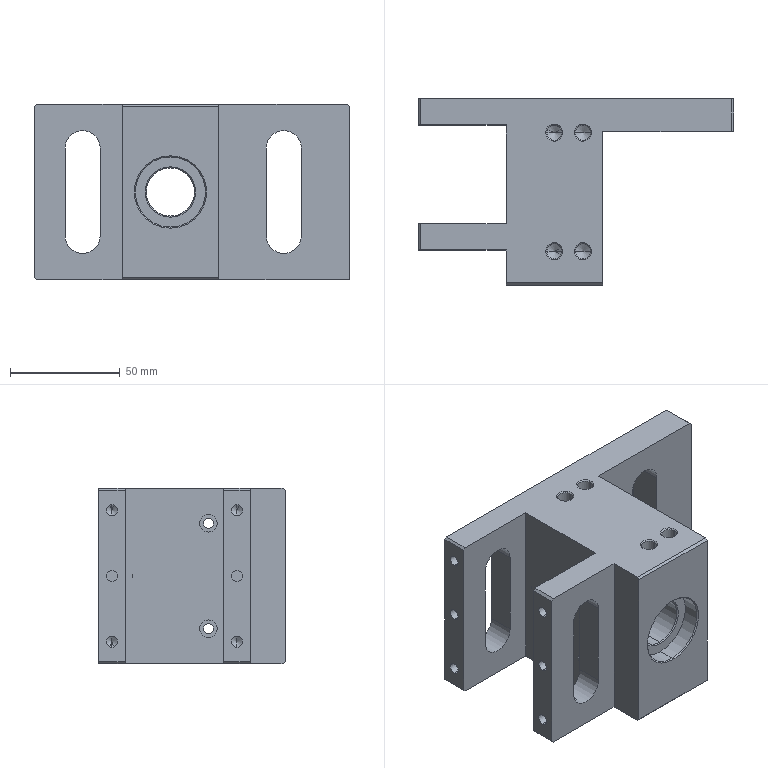Part | STEP file | longitudinal seal bearing seat 3_SUS304 | 1 solid | 142 faces | box 143.7 x 85 x 80 mm | volume 360424 mm3 | cylinder 59 | cone 50 | plane 33 | commonest cylinder face diameters 5 x12 6.8 x12 16 x9 3.3 x8 4.5 x4 8 x4